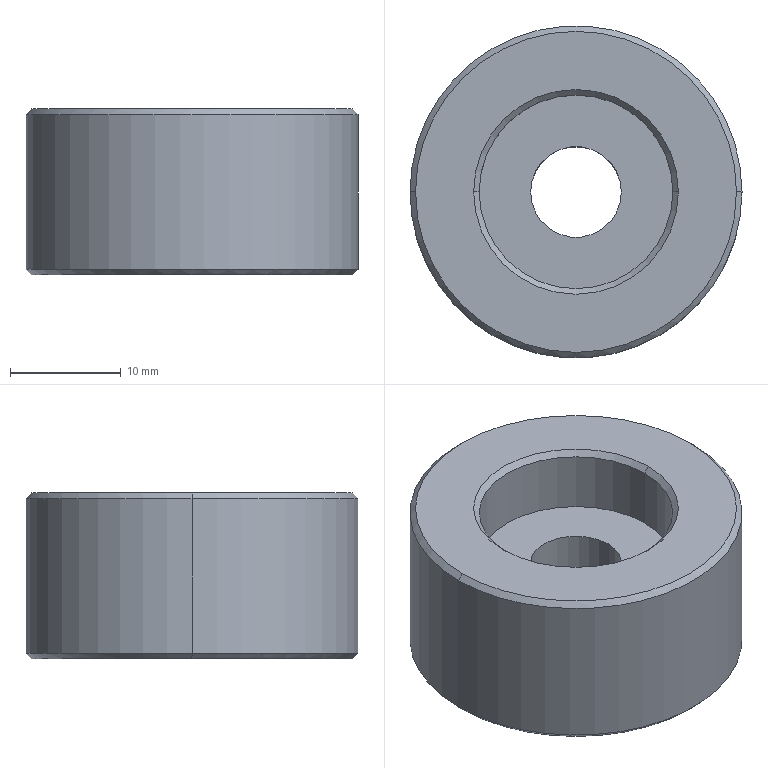Part | SolidWorks | features Chamfer 2, ICE 2, Extrusion 1 | 1 solid | 17 faces | box 30 x 30 x 15 mm | volume 8651 mm3 | cone 8 | cylinder 6 | plane 3 | commonest cylinder face diameters 8.2 x2 17.5 x2 30 x2
STEP:
#1=CARTESIAN_POINT('',(-14.5,0.,0.));
#2=VERTEX_POINT('',#1);
#3=CARTESIAN_POINT('',(14.5,0.,0.));
#4=VERTEX_POINT('',#3);
#5=CARTESIAN_POINT('',(0.,0.,0.));
#6=DIRECTION('',(0.,0.,-1.));
#7=DIRECTION('',(1.,0.,0.));
#8=AXIS2_PLACEMENT_3D('',#5,#6,#7);
#9=CIRCLE('',#8,14.5);
#10=EDGE_CURVE('',#2,#4,#9,.T.);
#11=ORIENTED_EDGE('',*,*,#10,.F.);
#12=CARTESIAN_POINT('',(-15.,0.,0.5));
#13=VERTEX_POINT('',#12);
#14=CARTESIAN_POINT('',(-15.,0.,0.5));
#15=DIRECTION('',(-0.7071,0.,0.7071));
#16=VECTOR('',#15,1000.);
#17=LINE('',#14,#16);
#18=EDGE_CURVE('',#2,#13,#17,.T.);
#19=ORIENTED_EDGE('',*,*,#18,.T.);
#20=CARTESIAN_POINT('',(15.,0.,0.5));
#21=VERTEX_POINT('',#20);
#22=CARTESIAN_POINT('',(0.,0.,0.5));
#23=DIRECTION('',(0.,0.,1.));
#24=DIRECTION('',(1.,0.,0.));
#25=AXIS2_PLACEMENT_3D('',#22,#23,#24);
#26=CIRCLE('',#25,15.);
#27=EDGE_CURVE('',#21,#13,#26,.T.);
#28=ORIENTED_EDGE('',*,*,#27,.F.);
#29=CARTESIAN_POINT('',(15.,0.,0.5));
#30=DIRECTION('',(0.7071,0.,0.7071));
#31=VECTOR('',#30,1000.);
#32=LINE('',#29,#31);
#33=EDGE_CURVE('',#4,#21,#32,.T.);
#34=ORIENTED_EDGE('',*,*,#33,.F.);
#35=EDGE_LOOP('',(#11,#19,#28,#34));
#36=FACE_OUTER_BOUND('',#35,.T.);
#37=CARTESIAN_POINT('',(0.,0.,0.5));
#38=DIRECTION('',(0.,0.,1.));
#39=DIRECTION('',(1.,0.,0.));
#40=AXIS2_PLACEMENT_3D('',#37,#38,#39);
#41=CONICAL_SURFACE('',#40,15.,0.7854);
#42=ADVANCED_FACE('',(#36),#41,.T.);
#43=CARTESIAN_POINT('',(14.5,0.,15.));
#44=VERTEX_POINT('',#43);
#45=CARTESIAN_POINT('',(-14.5,0.,15.));
#46=VERTEX_POINT('',#45);
#47=CARTESIAN_POINT('',(0.,0.,15.));
#48=DIRECTION('',(0.,0.,1.));
#49=DIRECTION('',(1.,0.,0.));
#50=AXIS2_PLACEMENT_3D('',#47,#48,#49);
#51=CIRCLE('',#50,14.5);
#52=EDGE_CURVE('',#44,#46,#51,.T.);
#53=ORIENTED_EDGE('',*,*,#52,.F.);
#54=CARTESIAN_POINT('',(15.,0.,14.5));
#55=VERTEX_POINT('',#54);
#56=CARTESIAN_POINT('',(14.5,0.,15.));
#57=DIRECTION('',(0.7071,0.,-0.7071));
#58=VECTOR('',#57,1000.);
#59=LINE('',#56,#58);
#60=EDGE_CURVE('',#44,#55,#59,.T.);
#61=ORIENTED_EDGE('',*,*,#60,.T.);
#62=CARTESIAN_POINT('',(-15.,0.,14.5));
#63=VERTEX_POINT('',#62);
#64=CARTESIAN_POINT('',(0.,0.,14.5));
#65=DIRECTION('',(0.,0.,-1.));
#66=DIRECTION('',(1.,0.,0.));
#67=AXIS2_PLACEMENT_3D('',#64,#65,#66);
#68=CIRCLE('',#67,15.);
#69=EDGE_CURVE('',#63,#55,#68,.T.);
#70=ORIENTED_EDGE('',*,*,#69,.F.);
#71=CARTESIAN_POINT('',(-14.5,0.,15.));
#72=DIRECTION('',(-0.7071,0.,-0.7071));
#73=VECTOR('',#72,1000.);
#74=LINE('',#71,#73);
#75=EDGE_CURVE('',#46,#63,#74,.T.);
#76=ORIENTED_EDGE('',*,*,#75,.F.);
#77=EDGE_LOOP('',(#53,#61,#70,#76));
#78=FACE_OUTER_BOUND('',#77,.T.);
#79=CARTESIAN_POINT('',(0.,0.,15.));
#80=DIRECTION('',(0.,0.,-1.));
#81=DIRECTION('',(-1.,0.,0.));
#82=AXIS2_PLACEMENT_3D('',#79,#80,#81);
#83=CONICAL_SURFACE('',#82,14.5,0.7854);
#84=ADVANCED_FACE('',(#78),#83,.T.);
#85=CARTESIAN_POINT('',(4.1,0.,0.5));
#86=VERTEX_POINT('',#85);
#87=CARTESIAN_POINT('',(-4.1,0.,0.5));
#88=VERTEX_POINT('',#87);
#89=CARTESIAN_POINT('',(0.,0.,0.5));
#90=DIRECTION('',(0.,0.,-1.));
#91=DIRECTION('',(1.,0.,0.));
#92=AXIS2_PLACEMENT_3D('',#89,#90,#91);
#93=CIRCLE('',#92,4.1);
#94=EDGE_CURVE('',#86,#88,#93,.T.);
#95=ORIENTED_EDGE('',*,*,#94,.F.);
#96=CARTESIAN_POINT('',(4.6,0.,0.));
#97=VERTEX_POINT('',#96);
#98=CARTESIAN_POINT('',(4.1,0.,0.5));
#99=DIRECTION('',(0.7071,0.,-0.7071));
#100=VECTOR('',#99,1000.);
#101=LINE('',#98,#100);
#102=EDGE_CURVE('',#86,#97,#101,.T.);
#103=ORIENTED_EDGE('',*,*,#102,.T.);
#104=CARTESIAN_POINT('',(-4.6,0.,0.));
#105=VERTEX_POINT('',#104);
#106=CARTESIAN_POINT('',(0.,0.,0.));
#107=DIRECTION('',(0.,0.,1.));
#108=DIRECTION('',(1.,0.,0.));
#109=AXIS2_PLACEMENT_3D('',#106,#107,#108);
#110=CIRCLE('',#109,4.6);
#111=EDGE_CURVE('',#105,#97,#110,.T.);
#112=ORIENTED_EDGE('',*,*,#111,.F.);
#113=CARTESIAN_POINT('',(-4.1,0.,0.5));
#114=DIRECTION('',(-0.7071,0.,-0.7071));
#115=VECTOR('',#114,1000.);
#116=LINE('',#113,#115);
#117=EDGE_CURVE('',#88,#105,#116,.T.);
#118=ORIENTED_EDGE('',*,*,#117,.F.);
#119=EDGE_LOOP('',(#95,#103,#112,#118));
#120=FACE_OUTER_BOUND('',#119,.T.);
#121=CARTESIAN_POINT('',(0.,0.,0.5));
#122=DIRECTION('',(0.,0.,-1.));
#123=DIRECTION('',(-1.,0.,0.));
#124=AXIS2_PLACEMENT_3D('',#121,#122,#123);
#125=CONICAL_SURFACE('',#124,4.1,0.7854);
#126=ADVANCED_FACE('',(#120),#125,.F.);
#127=CARTESIAN_POINT('',(-8.75,0.,14.5));
#128=VERTEX_POINT('',#127);
#129=CARTESIAN_POINT('',(8.75,0.,14.5));
#130=VERTEX_POINT('',#129);
#131=CARTESIAN_POINT('',(0.,0.,14.5));
#132=DIRECTION('',(0.,0.,1.));
#133=DIRECTION('',(1.,0.,0.));
#134=AXIS2_PLACEMENT_3D('',#131,#132,#133);
#135=CIRCLE('',#134,8.75);
#136=EDGE_CURVE('',#128,#130,#135,.T.);
#137=ORIENTED_EDGE('',*,*,#136,.F.);
#138=CARTESIAN_POINT('',(-9.25,0.,15.));
#139=VERTEX_POINT('',#138);
#140=CARTESIAN_POINT('',(-8.75,0.,14.5));
#141=DIRECTION('',(-0.7071,0.,0.7071));
#142=VECTOR('',#141,1000.);
#143=LINE('',#140,#142);
#144=EDGE_CURVE('',#128,#139,#143,.T.);
#145=ORIENTED_EDGE('',*,*,#144,.T.);
#146=CARTESIAN_POINT('',(9.25,0.,15.));
#147=VERTEX_POINT('',#146);
#148=CARTESIAN_POINT('',(0.,0.,15.));
#149=DIRECTION('',(0.,0.,-1.));
#150=DIRECTION('',(1.,0.,0.));
#151=AXIS2_PLACEMENT_3D('',#148,#149,#150);
#152=CIRCLE('',#151,9.25);
#153=EDGE_CURVE('',#147,#139,#152,.T.);
#154=ORIENTED_EDGE('',*,*,#153,.F.);
#155=CARTESIAN_POINT('',(8.75,0.,14.5));
#156=DIRECTION('',(0.7071,0.,0.7071));
#157=VECTOR('',#156,1000.);
#158=LINE('',#155,#157);
#159=EDGE_CURVE('',#130,#147,#158,.T.);
#160=ORIENTED_EDGE('',*,*,#159,.F.);
#161=EDGE_LOOP('',(#137,#145,#154,#160));
#162=FACE_OUTER_BOUND('',#161,.T.);
#163=CARTESIAN_POINT('',(0.,0.,14.5));
#164=DIRECTION('',(0.,0.,1.));
#165=DIRECTION('',(1.,0.,0.));
#166=AXIS2_PLACEMENT_3D('',#163,#164,#165);
#167=CONICAL_SURFACE('',#166,8.75,0.7854);
#168=ADVANCED_FACE('',(#162),#167,.F.);
#169=CARTESIAN_POINT('',(-8.75,0.,9.));
#170=VERTEX_POINT('',#169);
#171=CARTESIAN_POINT('',(8.75,0.,9.));
#172=VERTEX_POINT('',#171);
#173=CARTESIAN_POINT('',(0.,0.,9.));
#174=DIRECTION('',(0.,0.,1.));
#175=DIRECTION('',(1.,0.,0.));
#176=AXIS2_PLACEMENT_3D('',#173,#174,#175);
#177=CIRCLE('',#176,8.75);
#178=EDGE_CURVE('',#170,#172,#177,.T.);
#179=ORIENTED_EDGE('',*,*,#178,.F.);
#180=CARTESIAN_POINT('',(-8.75,0.,9.));
#181=DIRECTION('',(0.,0.,1.));
#182=VECTOR('',#181,1000.);
#183=LINE('',#180,#182);
#184=EDGE_CURVE('',#170,#128,#183,.T.);
#185=ORIENTED_EDGE('',*,*,#184,.T.);
#186=ORIENTED_EDGE('',*,*,#136,.T.);
#187=CARTESIAN_POINT('',(8.75,0.,9.));
#188=DIRECTION('',(0.,0.,1.));
#189=VECTOR('',#188,1000.);
#190=LINE('',#187,#189);
#191=EDGE_CURVE('',#172,#130,#190,.T.);
#192=ORIENTED_EDGE('',*,*,#191,.F.);
#193=EDGE_LOOP('',(#179,#185,#186,#192));
#194=FACE_OUTER_BOUND('',#193,.T.);
#195=CARTESIAN_POINT('',(0.,0.,9.));
#196=DIRECTION('',(0.,0.,1.));
#197=DIRECTION('',(1.,0.,0.));
#198=AXIS2_PLACEMENT_3D('',#195,#196,#197);
#199=CYLINDRICAL_SURFACE('',#198,8.75);
#200=ADVANCED_FACE('',(#194),#199,.F.);
#201=ORIENTED_EDGE('',*,*,#69,.T.);
#202=CARTESIAN_POINT('',(15.,0.,15.));
#203=DIRECTION('',(0.,0.,-1.));
#204=VECTOR('',#203,1000.);
#205=LINE('',#202,#204);
#206=EDGE_CURVE('',#55,#21,#205,.T.);
#207=ORIENTED_EDGE('',*,*,#206,.T.);
#208=ORIENTED_EDGE('',*,*,#27,.T.);
#209=CARTESIAN_POINT('',(-15.,0.,15.));
#210=DIRECTION('',(0.,0.,-1.));
#211=VECTOR('',#210,1000.);
#212=LINE('',#209,#211);
#213=EDGE_CURVE('',#63,#13,#212,.T.);
#214=ORIENTED_EDGE('',*,*,#213,.F.);
#215=EDGE_LOOP('',(#201,#207,#208,#214));
#216=FACE_OUTER_BOUND('',#215,.T.);
#217=CARTESIAN_POINT('',(0.,0.,15.));
#218=DIRECTION('',(0.,0.,-1.));
#219=DIRECTION('',(-1.,0.,0.));
#220=AXIS2_PLACEMENT_3D('',#217,#218,#219);
#221=CYLINDRICAL_SURFACE('',#220,15.);
#222=ADVANCED_FACE('',(#216),#221,.T.);
#223=CARTESIAN_POINT('',(4.1,0.,9.));
#224=VERTEX_POINT('',#223);
#225=CARTESIAN_POINT('',(-4.1,0.,9.));
#226=VERTEX_POINT('',#225);
#227=CARTESIAN_POINT('',(0.,0.,9.));
#228=DIRECTION('',(0.,0.,-1.));
#229=DIRECTION('',(1.,0.,0.));
#230=AXIS2_PLACEMENT_3D('',#227,#228,#229);
#231=CIRCLE('',#230,4.1);
#232=EDGE_CURVE('',#224,#226,#231,.T.);
#233=ORIENTED_EDGE('',*,*,#232,.F.);
#234=CARTESIAN_POINT('',(4.1,0.,50.));
#235=DIRECTION('',(0.,0.,-1.));
#236=VECTOR('',#235,1000.);
#237=LINE('',#234,#236);
#238=EDGE_CURVE('',#224,#86,#237,.T.);
#239=ORIENTED_EDGE('',*,*,#238,.T.);
#240=ORIENTED_EDGE('',*,*,#94,.T.);
#241=CARTESIAN_POINT('',(-4.1,0.,50.));
#242=DIRECTION('',(0.,0.,-1.));
#243=VECTOR('',#242,1000.);
#244=LINE('',#241,#243);
#245=EDGE_CURVE('',#226,#88,#244,.T.);
#246=ORIENTED_EDGE('',*,*,#245,.F.);
#247=EDGE_LOOP('',(#233,#239,#240,#246));
#248=FACE_OUTER_BOUND('',#247,.T.);
#249=CARTESIAN_POINT('',(0.,0.,50.));
#250=DIRECTION('',(0.,0.,-1.));
#251=DIRECTION('',(-1.,0.,0.));
#252=AXIS2_PLACEMENT_3D('',#249,#250,#251);
#253=CYLINDRICAL_SURFACE('',#252,4.1);
#254=ADVANCED_FACE('',(#248),#253,.F.);
#255=ORIENTED_EDGE('',*,*,#238,.F.);
#256=CARTESIAN_POINT('',(0.,0.,9.));
#257=DIRECTION('',(0.,0.,-1.));
#258=DIRECTION('',(1.,0.,0.));
#259=AXIS2_PLACEMENT_3D('',#256,#257,#258);
#260=CIRCLE('',#259,4.1);
#261=EDGE_CURVE('',#226,#224,#260,.T.);
#262=ORIENTED_EDGE('',*,*,#261,.F.);
#263=ORIENTED_EDGE('',*,*,#245,.T.);
#264=CARTESIAN_POINT('',(0.,0.,0.5));
#265=DIRECTION('',(0.,0.,-1.));
#266=DIRECTION('',(1.,0.,0.));
#267=AXIS2_PLACEMENT_3D('',#264,#265,#266);
#268=CIRCLE('',#267,4.1);
#269=EDGE_CURVE('',#88,#86,#268,.T.);
#270=ORIENTED_EDGE('',*,*,#269,.T.);
#271=EDGE_LOOP('',(#255,#262,#263,#270));
#272=FACE_OUTER_BOUND('',#271,.T.);
#273=CARTESIAN_POINT('',(0.,0.,50.));
#274=DIRECTION('',(0.,0.,-1.));
#275=DIRECTION('',(-1.,0.,0.));
#276=AXIS2_PLACEMENT_3D('',#273,#274,#275);
#277=CYLINDRICAL_SURFACE('',#276,4.1);
#278=ADVANCED_FACE('',(#272),#277,.F.);
#279=ORIENTED_EDGE('',*,*,#206,.F.);
#280=CARTESIAN_POINT('',(0.,0.,14.5));
#281=DIRECTION('',(0.,0.,-1.));
#282=DIRECTION('',(1.,0.,0.));
#283=AXIS2_PLACEMENT_3D('',#280,#281,#282);
#284=CIRCLE('',#283,15.);
#285=EDGE_CURVE('',#55,#63,#284,.T.);
#286=ORIENTED_EDGE('',*,*,#285,.T.);
#287=ORIENTED_EDGE('',*,*,#213,.T.);
#288=CARTESIAN_POINT('',(0.,0.,0.5));
#289=DIRECTION('',(0.,0.,1.));
#290=DIRECTION('',(1.,0.,0.));
#291=AXIS2_PLACEMENT_3D('',#288,#289,#290);
#292=CIRCLE('',#291,15.);
#293=EDGE_CURVE('',#13,#21,#292,.T.);
#294=ORIENTED_EDGE('',*,*,#293,.T.);
#295=EDGE_LOOP('',(#279,#286,#287,#294));
#296=FACE_OUTER_BOUND('',#295,.T.);
#297=CARTESIAN_POINT('',(0.,0.,15.));
#298=DIRECTION('',(0.,0.,-1.));
#299=DIRECTION('',(-1.,0.,0.));
#300=AXIS2_PLACEMENT_3D('',#297,#298,#299);
#301=CYLINDRICAL_SURFACE('',#300,15.);
#302=ADVANCED_FACE('',(#296),#301,.T.);
#303=CARTESIAN_POINT('',(0.,0.,15.));
#304=DIRECTION('',(0.,0.,1.));
#305=DIRECTION('',(1.,0.,0.));
#306=AXIS2_PLACEMENT_3D('',#303,#304,#305);
#307=CIRCLE('',#306,14.5);
#308=EDGE_CURVE('',#46,#44,#307,.T.);
#309=ORIENTED_EDGE('',*,*,#308,.T.);
#310=ORIENTED_EDGE('',*,*,#52,.T.);
#311=EDGE_LOOP('',(#309,#310));
#312=FACE_OUTER_BOUND('',#311,.T.);
#313=ORIENTED_EDGE('',*,*,#153,.T.);
#314=CARTESIAN_POINT('',(0.,0.,15.));
#315=DIRECTION('',(0.,0.,-1.));
#316=DIRECTION('',(1.,0.,0.));
#317=AXIS2_PLACEMENT_3D('',#314,#315,#316);
#318=CIRCLE('',#317,9.25);
#319=EDGE_CURVE('',#139,#147,#318,.T.);
#320=ORIENTED_EDGE('',*,*,#319,.T.);
#321=EDGE_LOOP('',(#313,#320));
#322=FACE_BOUND('',#321,.T.);
#323=CARTESIAN_POINT('',(0.,0.,15.));
#324=DIRECTION('',(0.,0.,1.));
#325=DIRECTION('',(1.,0.,0.));
#326=AXIS2_PLACEMENT_3D('',#323,#324,#325);
#327=PLANE('',#326);
#328=ADVANCED_FACE('',(#312,#322),#327,.T.);
#329=ORIENTED_EDGE('',*,*,#111,.T.);
#330=CARTESIAN_POINT('',(0.,0.,0.));
#331=DIRECTION('',(0.,0.,1.));
#332=DIRECTION('',(1.,0.,0.));
#333=AXIS2_PLACEMENT_3D('',#330,#331,#332);
#334=CIRCLE('',#333,4.6);
#335=EDGE_CURVE('',#97,#105,#334,.T.);
#336=ORIENTED_EDGE('',*,*,#335,.T.);
#337=EDGE_LOOP('',(#329,#336));
#338=FACE_BOUND('',#337,.T.);
#339=CARTESIAN_POINT('',(0.,0.,0.));
#340=DIRECTION('',(0.,0.,-1.));
#341=DIRECTION('',(1.,0.,0.));
#342=AXIS2_PLACEMENT_3D('',#339,#340,#341);
#343=CIRCLE('',#342,14.5);
#344=EDGE_CURVE('',#4,#2,#343,.T.);
#345=ORIENTED_EDGE('',*,*,#344,.T.);
#346=ORIENTED_EDGE('',*,*,#10,.T.);
#347=EDGE_LOOP('',(#345,#346));
#348=FACE_OUTER_BOUND('',#347,.T.);
#349=CARTESIAN_POINT('',(0.,0.,0.));
#350=DIRECTION('',(0.,0.,1.));
#351=DIRECTION('',(1.,0.,0.));
#352=AXIS2_PLACEMENT_3D('',#349,#350,#351);
#353=PLANE('',#352);
#354=ADVANCED_FACE('',(#338,#348),#353,.F.);
#355=CARTESIAN_POINT('',(0.,0.,9.));
#356=DIRECTION('',(0.,0.,1.));
#357=DIRECTION('',(1.,0.,0.));
#358=AXIS2_PLACEMENT_3D('',#355,#356,#357);
#359=CIRCLE('',#358,8.75);
#360=EDGE_CURVE('',#172,#170,#359,.T.);
#361=ORIENTED_EDGE('',*,*,#360,.T.);
#362=ORIENTED_EDGE('',*,*,#178,.T.);
#363=EDGE_LOOP('',(#361,#362));
#364=FACE_OUTER_BOUND('',#363,.T.);
#365=ORIENTED_EDGE('',*,*,#261,.T.);
#366=ORIENTED_EDGE('',*,*,#232,.T.);
#367=EDGE_LOOP('',(#365,#366));
#368=FACE_BOUND('',#367,.T.);
#369=CARTESIAN_POINT('',(0.,0.,9.));
#370=DIRECTION('',(0.,0.,1.));
#371=DIRECTION('',(1.,0.,0.));
#372=AXIS2_PLACEMENT_3D('',#369,#370,#371);
#373=PLANE('',#372);
#374=ADVANCED_FACE('',(#364,#368),#373,.T.);
#375=ORIENTED_EDGE('',*,*,#184,.F.);
#376=ORIENTED_EDGE('',*,*,#360,.F.);
#377=ORIENTED_EDGE('',*,*,#191,.T.);
#378=CARTESIAN_POINT('',(0.,0.,14.5));
#379=DIRECTION('',(0.,0.,1.));
#380=DIRECTION('',(1.,0.,0.));
#381=AXIS2_PLACEMENT_3D('',#378,#379,#380);
#382=CIRCLE('',#381,8.75);
#383=EDGE_CURVE('',#130,#128,#382,.T.);
#384=ORIENTED_EDGE('',*,*,#383,.T.);
#385=EDGE_LOOP('',(#375,#376,#377,#384));
#386=FACE_OUTER_BOUND('',#385,.T.);
#387=CARTESIAN_POINT('',(0.,0.,9.));
#388=DIRECTION('',(0.,0.,1.));
#389=DIRECTION('',(1.,0.,0.));
#390=AXIS2_PLACEMENT_3D('',#387,#388,#389);
#391=CYLINDRICAL_SURFACE('',#390,8.75);
#392=ADVANCED_FACE('',(#386),#391,.F.);
#393=ORIENTED_EDGE('',*,*,#144,.F.);
#394=ORIENTED_EDGE('',*,*,#383,.F.);
#395=ORIENTED_EDGE('',*,*,#159,.T.);
#396=ORIENTED_EDGE('',*,*,#319,.F.);
#397=EDGE_LOOP('',(#393,#394,#395,#396));
#398=FACE_OUTER_BOUND('',#397,.T.);
#399=CARTESIAN_POINT('',(0.,0.,14.5));
#400=DIRECTION('',(0.,0.,1.));
#401=DIRECTION('',(1.,0.,0.));
#402=AXIS2_PLACEMENT_3D('',#399,#400,#401);
#403=CONICAL_SURFACE('',#402,8.75,0.7854);
#404=ADVANCED_FACE('',(#398),#403,.F.);
#405=ORIENTED_EDGE('',*,*,#102,.F.);
#406=ORIENTED_EDGE('',*,*,#269,.F.);
#407=ORIENTED_EDGE('',*,*,#117,.T.);
#408=ORIENTED_EDGE('',*,*,#335,.F.);
#409=EDGE_LOOP('',(#405,#406,#407,#408));
#410=FACE_OUTER_BOUND('',#409,.T.);
#411=CARTESIAN_POINT('',(0.,0.,0.5));
#412=DIRECTION('',(0.,0.,-1.));
#413=DIRECTION('',(-1.,0.,0.));
#414=AXIS2_PLACEMENT_3D('',#411,#412,#413);
#415=CONICAL_SURFACE('',#414,4.1,0.7854);
#416=ADVANCED_FACE('',(#410),#415,.F.);
#417=ORIENTED_EDGE('',*,*,#60,.F.);
#418=ORIENTED_EDGE('',*,*,#308,.F.);
#419=ORIENTED_EDGE('',*,*,#75,.T.);
#420=ORIENTED_EDGE('',*,*,#285,.F.);
#421=EDGE_LOOP('',(#417,#418,#419,#420));
#422=FACE_OUTER_BOUND('',#421,.T.);
#423=CARTESIAN_POINT('',(0.,0.,15.));
#424=DIRECTION('',(0.,0.,-1.));
#425=DIRECTION('',(-1.,0.,0.));
#426=AXIS2_PLACEMENT_3D('',#423,#424,#425);
#427=CONICAL_SURFACE('',#426,14.5,0.7854);
#428=ADVANCED_FACE('',(#422),#427,.T.);
#429=ORIENTED_EDGE('',*,*,#18,.F.);
#430=ORIENTED_EDGE('',*,*,#344,.F.);
#431=ORIENTED_EDGE('',*,*,#33,.T.);
#432=ORIENTED_EDGE('',*,*,#293,.F.);
#433=EDGE_LOOP('',(#429,#430,#431,#432));
#434=FACE_OUTER_BOUND('',#433,.T.);
#435=CARTESIAN_POINT('',(0.,0.,0.5));
#436=DIRECTION('',(0.,0.,1.));
#437=DIRECTION('',(1.,0.,0.));
#438=AXIS2_PLACEMENT_3D('',#435,#436,#437);
#439=CONICAL_SURFACE('',#438,15.,0.7854);
#440=ADVANCED_FACE('',(#434),#439,.T.);
#441=CLOSED_SHELL('',(#42,#84,#126,#168,#200,#222,#254,#278,#302,#328,#354,#374,#392,#404,#416,#428,#440));
#442=MANIFOLD_SOLID_BREP('',#441);
#443=CARTESIAN_POINT('',(0.,0.,0.));
#444=DIRECTION('',(0.,0.,1.));
#445=DIRECTION('',(1.,0.,0.));
#446=AXIS2_PLACEMENT_3D('',#443,#444,#445);
#447=(LENGTH_UNIT()NAMED_UNIT(*)SI_UNIT(.MILLI.,.METRE.));
#448=UNCERTAINTY_MEASURE_WITH_UNIT(LENGTH_MEASURE(0.00001),#447,'','');
#449=(NAMED_UNIT(*)PLANE_ANGLE_UNIT()SI_UNIT($,.RADIAN.));
#450=(NAMED_UNIT(*)SI_UNIT($,.STERADIAN.)SOLID_ANGLE_UNIT());
#451=(GEOMETRIC_REPRESENTATION_CONTEXT(3)GLOBAL_UNCERTAINTY_ASSIGNED_CONTEXT((#448))GLOBAL_UNIT_ASSIGNED_CONTEXT((#447,#449,#450))REPRESENTATION_CONTEXT('',''));
#452=ADVANCED_BREP_SHAPE_REPRESENTATION('',(#442,#446),#451);